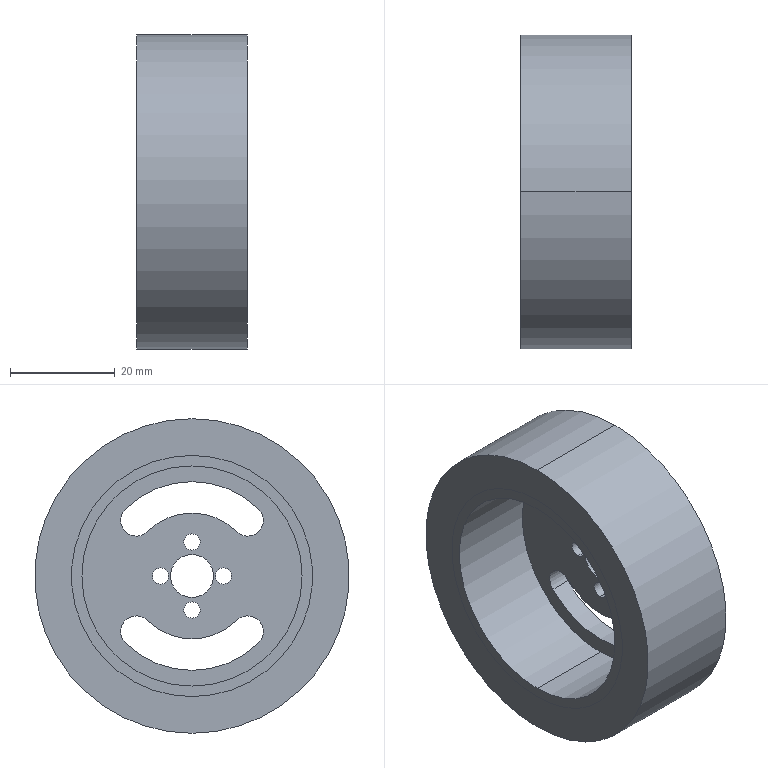Part | SolidWorks | features BaseBody 2 | 2 solids | 35 faces | box 21 x 60 x 60 mm | volume 34134 mm3 | cylinder 30 | plane 5 | commonest cylinder face diameters 3.1 x8 6 x6 46 x4 24 x3 36 x3 8.2 x2
STEP:
#1=CARTESIAN_POINT('',(39.982,27.528,21.886));
#2=VERTEX_POINT('',#1);
#3=CARTESIAN_POINT('',(18.982,27.528,21.886));
#4=VERTEX_POINT('',#3);
#5=CARTESIAN_POINT('',(39.982,27.528,21.886));
#6=DIRECTION('',(-1.,0.,0.));
#7=VECTOR('',#6,1000.);
#8=LINE('',#5,#7);
#9=EDGE_CURVE('',#2,#4,#8,.T.);
#10=ORIENTED_EDGE('',*,*,#9,.F.);
#11=CARTESIAN_POINT('',(39.982,27.528,67.886));
#12=VERTEX_POINT('',#11);
#13=CARTESIAN_POINT('',(39.982,27.528,44.886));
#14=DIRECTION('',(1.,0.,0.));
#15=DIRECTION('',(0.,0.,-1.));
#16=AXIS2_PLACEMENT_3D('',#13,#14,#15);
#17=CIRCLE('',#16,23.);
#18=EDGE_CURVE('',#2,#12,#17,.T.);
#19=ORIENTED_EDGE('',*,*,#18,.T.);
#20=CARTESIAN_POINT('',(18.982,27.528,67.886));
#21=VERTEX_POINT('',#20);
#22=CARTESIAN_POINT('',(39.982,27.528,67.886));
#23=DIRECTION('',(-1.,0.,0.));
#24=VECTOR('',#23,1000.);
#25=LINE('',#22,#24);
#26=EDGE_CURVE('',#12,#21,#25,.T.);
#27=ORIENTED_EDGE('',*,*,#26,.T.);
#28=CARTESIAN_POINT('',(18.982,27.528,44.886));
#29=DIRECTION('',(1.,0.,0.));
#30=DIRECTION('',(0.,0.,-1.));
#31=AXIS2_PLACEMENT_3D('',#28,#29,#30);
#32=CIRCLE('',#31,23.);
#33=EDGE_CURVE('',#4,#21,#32,.T.);
#34=ORIENTED_EDGE('',*,*,#33,.F.);
#35=EDGE_LOOP('',(#10,#19,#27,#34));
#36=FACE_OUTER_BOUND('',#35,.T.);
#37=CARTESIAN_POINT('',(39.982,27.528,44.886));
#38=DIRECTION('',(-1.,0.,0.));
#39=DIRECTION('',(0.,0.,1.));
#40=AXIS2_PLACEMENT_3D('',#37,#38,#39);
#41=CYLINDRICAL_SURFACE('',#40,23.);
#42=ADVANCED_FACE('',(#36),#41,.F.);
#43=CARTESIAN_POINT('',(39.982,27.528,14.886));
#44=VERTEX_POINT('',#43);
#45=CARTESIAN_POINT('',(18.982,27.528,14.886));
#46=VERTEX_POINT('',#45);
#47=CARTESIAN_POINT('',(39.982,27.528,14.886));
#48=DIRECTION('',(-1.,0.,0.));
#49=VECTOR('',#48,1000.);
#50=LINE('',#47,#49);
#51=EDGE_CURVE('',#44,#46,#50,.T.);
#52=ORIENTED_EDGE('',*,*,#51,.F.);
#53=CARTESIAN_POINT('',(39.982,27.528,74.886));
#54=VERTEX_POINT('',#53);
#55=CARTESIAN_POINT('',(39.982,27.528,44.886));
#56=DIRECTION('',(1.,0.,0.));
#57=DIRECTION('',(0.,0.,-1.));
#58=AXIS2_PLACEMENT_3D('',#55,#56,#57);
#59=CIRCLE('',#58,30.);
#60=EDGE_CURVE('',#54,#44,#59,.T.);
#61=ORIENTED_EDGE('',*,*,#60,.F.);
#62=CARTESIAN_POINT('',(18.982,27.528,74.886));
#63=VERTEX_POINT('',#62);
#64=CARTESIAN_POINT('',(39.982,27.528,74.886));
#65=DIRECTION('',(-1.,0.,0.));
#66=VECTOR('',#65,1000.);
#67=LINE('',#64,#66);
#68=EDGE_CURVE('',#54,#63,#67,.T.);
#69=ORIENTED_EDGE('',*,*,#68,.T.);
#70=CARTESIAN_POINT('',(18.982,27.528,44.886));
#71=DIRECTION('',(1.,0.,0.));
#72=DIRECTION('',(0.,0.,-1.));
#73=AXIS2_PLACEMENT_3D('',#70,#71,#72);
#74=CIRCLE('',#73,30.);
#75=EDGE_CURVE('',#63,#46,#74,.T.);
#76=ORIENTED_EDGE('',*,*,#75,.T.);
#77=EDGE_LOOP('',(#52,#61,#69,#76));
#78=FACE_OUTER_BOUND('',#77,.T.);
#79=CARTESIAN_POINT('',(39.982,27.528,44.886));
#80=DIRECTION('',(-1.,0.,0.));
#81=DIRECTION('',(0.,0.,1.));
#82=AXIS2_PLACEMENT_3D('',#79,#80,#81);
#83=CYLINDRICAL_SURFACE('',#82,30.);
#84=ADVANCED_FACE('',(#78),#83,.T.);
#85=CARTESIAN_POINT('',(18.982,27.528,44.886));
#86=DIRECTION('',(1.,0.,0.));
#87=DIRECTION('',(0.,0.,-1.));
#88=AXIS2_PLACEMENT_3D('',#85,#86,#87);
#89=CIRCLE('',#88,23.);
#90=EDGE_CURVE('',#21,#4,#89,.T.);
#91=ORIENTED_EDGE('',*,*,#90,.T.);
#92=ORIENTED_EDGE('',*,*,#33,.T.);
#93=EDGE_LOOP('',(#91,#92));
#94=FACE_BOUND('',#93,.T.);
#95=ORIENTED_EDGE('',*,*,#75,.F.);
#96=CARTESIAN_POINT('',(18.982,27.528,44.886));
#97=DIRECTION('',(1.,0.,0.));
#98=DIRECTION('',(0.,0.,-1.));
#99=AXIS2_PLACEMENT_3D('',#96,#97,#98);
#100=CIRCLE('',#99,30.);
#101=EDGE_CURVE('',#46,#63,#100,.T.);
#102=ORIENTED_EDGE('',*,*,#101,.F.);
#103=EDGE_LOOP('',(#95,#102));
#104=FACE_OUTER_BOUND('',#103,.T.);
#105=CARTESIAN_POINT('',(18.982,27.528,44.886));
#106=DIRECTION('',(1.,0.,0.));
#107=DIRECTION('',(0.,1.,0.));
#108=AXIS2_PLACEMENT_3D('',#105,#106,#107);
#109=PLANE('',#108);
#110=ADVANCED_FACE('',(#94,#104),#109,.F.);
#111=CARTESIAN_POINT('',(39.982,27.528,44.886));
#112=DIRECTION('',(1.,0.,0.));
#113=DIRECTION('',(0.,0.,-1.));
#114=AXIS2_PLACEMENT_3D('',#111,#112,#113);
#115=CIRCLE('',#114,23.);
#116=EDGE_CURVE('',#12,#2,#115,.T.);
#117=ORIENTED_EDGE('',*,*,#116,.F.);
#118=ORIENTED_EDGE('',*,*,#18,.F.);
#119=EDGE_LOOP('',(#117,#118));
#120=FACE_BOUND('',#119,.T.);
#121=ORIENTED_EDGE('',*,*,#60,.T.);
#122=CARTESIAN_POINT('',(39.982,27.528,44.886));
#123=DIRECTION('',(1.,0.,0.));
#124=DIRECTION('',(0.,0.,-1.));
#125=AXIS2_PLACEMENT_3D('',#122,#123,#124);
#126=CIRCLE('',#125,30.);
#127=EDGE_CURVE('',#44,#54,#126,.T.);
#128=ORIENTED_EDGE('',*,*,#127,.T.);
#129=EDGE_LOOP('',(#121,#128));
#130=FACE_OUTER_BOUND('',#129,.T.);
#131=CARTESIAN_POINT('',(39.982,27.528,44.886));
#132=DIRECTION('',(1.,0.,0.));
#133=DIRECTION('',(0.,1.,0.));
#134=AXIS2_PLACEMENT_3D('',#131,#132,#133);
#135=PLANE('',#134);
#136=ADVANCED_FACE('',(#120,#130),#135,.T.);
#137=ORIENTED_EDGE('',*,*,#127,.F.);
#138=ORIENTED_EDGE('',*,*,#51,.T.);
#139=ORIENTED_EDGE('',*,*,#101,.T.);
#140=ORIENTED_EDGE('',*,*,#68,.F.);
#141=EDGE_LOOP('',(#137,#138,#139,#140));
#142=FACE_OUTER_BOUND('',#141,.T.);
#143=CARTESIAN_POINT('',(39.982,27.528,44.886));
#144=DIRECTION('',(-1.,0.,0.));
#145=DIRECTION('',(0.,0.,1.));
#146=AXIS2_PLACEMENT_3D('',#143,#144,#145);
#147=CYLINDRICAL_SURFACE('',#146,30.);
#148=ADVANCED_FACE('',(#142),#147,.T.);
#149=ORIENTED_EDGE('',*,*,#116,.T.);
#150=ORIENTED_EDGE('',*,*,#9,.T.);
#151=ORIENTED_EDGE('',*,*,#90,.F.);
#152=ORIENTED_EDGE('',*,*,#26,.F.);
#153=EDGE_LOOP('',(#149,#150,#151,#152));
#154=FACE_OUTER_BOUND('',#153,.T.);
#155=CARTESIAN_POINT('',(39.982,27.528,44.886));
#156=DIRECTION('',(-1.,0.,0.));
#157=DIRECTION('',(0.,0.,1.));
#158=AXIS2_PLACEMENT_3D('',#155,#156,#157);
#159=CYLINDRICAL_SURFACE('',#158,23.);
#160=ADVANCED_FACE('',(#154),#159,.F.);
#161=CLOSED_SHELL('',(#42,#84,#110,#136,#148,#160));
#162=MANIFOLD_SOLID_BREP('',#161);
#163=CARTESIAN_POINT('',(35.982,27.528,39.936));
#164=VERTEX_POINT('',#163);
#165=CARTESIAN_POINT('',(35.982,27.528,36.836));
#166=VERTEX_POINT('',#165);
#167=CARTESIAN_POINT('',(35.982,27.528,38.386));
#168=DIRECTION('',(-1.,0.,0.));
#169=DIRECTION('',(0.,0.,1.));
#170=AXIS2_PLACEMENT_3D('',#167,#168,#169);
#171=CIRCLE('',#170,1.55);
#172=EDGE_CURVE('',#164,#166,#171,.T.);
#173=ORIENTED_EDGE('',*,*,#172,.F.);
#174=CARTESIAN_POINT('',(35.982,27.528,38.386));
#175=DIRECTION('',(-1.,0.,0.));
#176=DIRECTION('',(0.,0.,1.));
#177=AXIS2_PLACEMENT_3D('',#174,#175,#176);
#178=CIRCLE('',#177,1.55);
#179=EDGE_CURVE('',#166,#164,#178,.T.);
#180=ORIENTED_EDGE('',*,*,#179,.F.);
#181=EDGE_LOOP('',(#173,#180));
#182=FACE_BOUND('',#181,.T.);
#183=CARTESIAN_POINT('',(35.982,21.528,46.436));
#184=VERTEX_POINT('',#183);
#185=CARTESIAN_POINT('',(35.982,21.528,43.336));
#186=VERTEX_POINT('',#185);
#187=CARTESIAN_POINT('',(35.982,21.528,44.886));
#188=DIRECTION('',(-1.,0.,0.));
#189=DIRECTION('',(0.,0.,-1.));
#190=AXIS2_PLACEMENT_3D('',#187,#188,#189);
#191=CIRCLE('',#190,1.55);
#192=EDGE_CURVE('',#184,#186,#191,.T.);
#193=ORIENTED_EDGE('',*,*,#192,.F.);
#194=CARTESIAN_POINT('',(35.982,21.528,44.886));
#195=DIRECTION('',(-1.,0.,0.));
#196=DIRECTION('',(0.,0.,-1.));
#197=AXIS2_PLACEMENT_3D('',#194,#195,#196);
#198=CIRCLE('',#197,1.55);
#199=EDGE_CURVE('',#186,#184,#198,.T.);
#200=ORIENTED_EDGE('',*,*,#199,.F.);
#201=EDGE_LOOP('',(#193,#200));
#202=FACE_BOUND('',#201,.T.);
#203=CARTESIAN_POINT('',(35.982,27.528,52.936));
#204=VERTEX_POINT('',#203);
#205=CARTESIAN_POINT('',(35.982,27.528,49.836));
#206=VERTEX_POINT('',#205);
#207=CARTESIAN_POINT('',(35.982,27.528,51.386));
#208=DIRECTION('',(-1.,0.,0.));
#209=DIRECTION('',(0.,0.,-1.));
#210=AXIS2_PLACEMENT_3D('',#207,#208,#209);
#211=CIRCLE('',#210,1.55);
#212=EDGE_CURVE('',#204,#206,#211,.T.);
#213=ORIENTED_EDGE('',*,*,#212,.F.);
#214=CARTESIAN_POINT('',(35.982,27.528,51.386));
#215=DIRECTION('',(-1.,0.,0.));
#216=DIRECTION('',(0.,0.,-1.));
#217=AXIS2_PLACEMENT_3D('',#214,#215,#216);
#218=CIRCLE('',#217,1.55);
#219=EDGE_CURVE('',#206,#204,#218,.T.);
#220=ORIENTED_EDGE('',*,*,#219,.F.);
#221=EDGE_LOOP('',(#213,#220));
#222=FACE_BOUND('',#221,.T.);
#223=CARTESIAN_POINT('',(35.982,33.528,46.436));
#224=VERTEX_POINT('',#223);
#225=CARTESIAN_POINT('',(35.982,33.528,43.336));
#226=VERTEX_POINT('',#225);
#227=CARTESIAN_POINT('',(35.982,33.528,44.886));
#228=DIRECTION('',(-1.,0.,0.));
#229=DIRECTION('',(0.,0.,1.));
#230=AXIS2_PLACEMENT_3D('',#227,#228,#229);
#231=CIRCLE('',#230,1.55);
#232=EDGE_CURVE('',#224,#226,#231,.T.);
#233=ORIENTED_EDGE('',*,*,#232,.F.);
#234=CARTESIAN_POINT('',(35.982,33.528,44.886));
#235=DIRECTION('',(-1.,0.,0.));
#236=DIRECTION('',(0.,0.,1.));
#237=AXIS2_PLACEMENT_3D('',#234,#235,#236);
#238=CIRCLE('',#237,1.55);
#239=EDGE_CURVE('',#226,#224,#238,.T.);
#240=ORIENTED_EDGE('',*,*,#239,.F.);
#241=EDGE_LOOP('',(#233,#240));
#242=FACE_BOUND('',#241,.T.);
#243=CARTESIAN_POINT('',(35.982,27.528,48.986));
#244=VERTEX_POINT('',#243);
#245=CARTESIAN_POINT('',(35.982,27.528,40.786));
#246=VERTEX_POINT('',#245);
#247=CARTESIAN_POINT('',(35.982,27.528,44.886));
#248=DIRECTION('',(-1.,0.,0.));
#249=DIRECTION('',(0.,0.,-1.));
#250=AXIS2_PLACEMENT_3D('',#247,#248,#249);
#251=CIRCLE('',#250,4.1);
#252=EDGE_CURVE('',#244,#246,#251,.T.);
#253=ORIENTED_EDGE('',*,*,#252,.F.);
#254=CARTESIAN_POINT('',(35.982,27.528,44.886));
#255=DIRECTION('',(-1.,0.,0.));
#256=DIRECTION('',(0.,0.,-1.));
#257=AXIS2_PLACEMENT_3D('',#254,#255,#256);
#258=CIRCLE('',#257,4.1);
#259=EDGE_CURVE('',#246,#244,#258,.T.);
#260=ORIENTED_EDGE('',*,*,#259,.F.);
#261=EDGE_LOOP('',(#253,#260));
#262=FACE_BOUND('',#261,.T.);
#263=CARTESIAN_POINT('',(35.982,19.043,36.401));
#264=VERTEX_POINT('',#263);
#265=CARTESIAN_POINT('',(35.982,36.014,36.401));
#266=VERTEX_POINT('',#265);
#267=CARTESIAN_POINT('',(35.982,27.528,44.886));
#268=DIRECTION('',(1.,0.,0.));
#269=DIRECTION('',(0.,0.,-1.));
#270=AXIS2_PLACEMENT_3D('',#267,#268,#269);
#271=CIRCLE('',#270,12.);
#272=EDGE_CURVE('',#264,#266,#271,.T.);
#273=ORIENTED_EDGE('',*,*,#272,.F.);
#274=CARTESIAN_POINT('',(35.982,16.922,37.28));
#275=VERTEX_POINT('',#274);
#276=CARTESIAN_POINT('',(35.982,16.922,34.28));
#277=DIRECTION('',(-1.,0.,0.));
#278=DIRECTION('',(0.,0.,-1.));
#279=AXIS2_PLACEMENT_3D('',#276,#277,#278);
#280=CIRCLE('',#279,3.);
#281=EDGE_CURVE('',#275,#264,#280,.T.);
#282=ORIENTED_EDGE('',*,*,#281,.F.);
#283=CARTESIAN_POINT('',(35.982,14.801,32.158));
#284=VERTEX_POINT('',#283);
#285=CARTESIAN_POINT('',(35.982,16.922,34.28));
#286=DIRECTION('',(-1.,0.,0.));
#287=DIRECTION('',(0.,0.,-1.));
#288=AXIS2_PLACEMENT_3D('',#285,#286,#287);
#289=CIRCLE('',#288,3.);
#290=EDGE_CURVE('',#284,#275,#289,.T.);
#291=ORIENTED_EDGE('',*,*,#290,.F.);
#292=CARTESIAN_POINT('',(35.982,40.256,32.158));
#293=VERTEX_POINT('',#292);
#294=CARTESIAN_POINT('',(35.982,27.528,44.886));
#295=DIRECTION('',(-1.,0.,0.));
#296=DIRECTION('',(0.,0.,-1.));
#297=AXIS2_PLACEMENT_3D('',#294,#295,#296);
#298=CIRCLE('',#297,18.);
#299=EDGE_CURVE('',#293,#284,#298,.T.);
#300=ORIENTED_EDGE('',*,*,#299,.F.);
#301=CARTESIAN_POINT('',(35.982,38.135,37.28));
#302=VERTEX_POINT('',#301);
#303=CARTESIAN_POINT('',(35.982,38.135,34.28));
#304=DIRECTION('',(-1.,0.,0.));
#305=DIRECTION('',(0.,0.,-1.));
#306=AXIS2_PLACEMENT_3D('',#303,#304,#305);
#307=CIRCLE('',#306,3.);
#308=EDGE_CURVE('',#302,#293,#307,.T.);
#309=ORIENTED_EDGE('',*,*,#308,.F.);
#310=CARTESIAN_POINT('',(35.982,38.135,34.28));
#311=DIRECTION('',(-1.,0.,0.));
#312=DIRECTION('',(0.,0.,-1.));
#313=AXIS2_PLACEMENT_3D('',#310,#311,#312);
#314=CIRCLE('',#313,3.);
#315=EDGE_CURVE('',#266,#302,#314,.T.);
#316=ORIENTED_EDGE('',*,*,#315,.F.);
#317=EDGE_LOOP('',(#273,#282,#291,#300,#309,#316));
#318=FACE_BOUND('',#317,.T.);
#319=CARTESIAN_POINT('',(35.982,19.043,53.372));
#320=VERTEX_POINT('',#319);
#321=CARTESIAN_POINT('',(35.982,14.801,57.614));
#322=VERTEX_POINT('',#321);
#323=CARTESIAN_POINT('',(35.982,16.922,55.493));
#324=DIRECTION('',(-1.,0.,0.));
#325=DIRECTION('',(0.,0.,1.));
#326=AXIS2_PLACEMENT_3D('',#323,#324,#325);
#327=CIRCLE('',#326,3.);
#328=EDGE_CURVE('',#320,#322,#327,.T.);
#329=ORIENTED_EDGE('',*,*,#328,.F.);
#330=CARTESIAN_POINT('',(35.982,27.528,56.886));
#331=VERTEX_POINT('',#330);
#332=CARTESIAN_POINT('',(35.982,27.528,44.886));
#333=DIRECTION('',(1.,0.,0.));
#334=DIRECTION('',(0.,0.,1.));
#335=AXIS2_PLACEMENT_3D('',#332,#333,#334);
#336=CIRCLE('',#335,12.);
#337=EDGE_CURVE('',#331,#320,#336,.T.);
#338=ORIENTED_EDGE('',*,*,#337,.F.);
#339=CARTESIAN_POINT('',(35.982,36.014,53.372));
#340=VERTEX_POINT('',#339);
#341=CARTESIAN_POINT('',(35.982,27.528,44.886));
#342=DIRECTION('',(1.,0.,0.));
#343=DIRECTION('',(0.,0.,1.));
#344=AXIS2_PLACEMENT_3D('',#341,#342,#343);
#345=CIRCLE('',#344,12.);
#346=EDGE_CURVE('',#340,#331,#345,.T.);
#347=ORIENTED_EDGE('',*,*,#346,.F.);
#348=CARTESIAN_POINT('',(35.982,40.256,57.614));
#349=VERTEX_POINT('',#348);
#350=CARTESIAN_POINT('',(35.982,38.135,55.493));
#351=DIRECTION('',(-1.,0.,0.));
#352=DIRECTION('',(0.,0.,1.));
#353=AXIS2_PLACEMENT_3D('',#350,#351,#352);
#354=CIRCLE('',#353,3.);
#355=EDGE_CURVE('',#349,#340,#354,.T.);
#356=ORIENTED_EDGE('',*,*,#355,.F.);
#357=CARTESIAN_POINT('',(35.982,27.528,62.886));
#358=VERTEX_POINT('',#357);
#359=CARTESIAN_POINT('',(35.982,27.528,44.886));
#360=DIRECTION('',(-1.,0.,0.));
#361=DIRECTION('',(0.,0.,1.));
#362=AXIS2_PLACEMENT_3D('',#359,#360,#361);
#363=CIRCLE('',#362,18.);
#364=EDGE_CURVE('',#358,#349,#363,.T.);
#365=ORIENTED_EDGE('',*,*,#364,.F.);
#366=CARTESIAN_POINT('',(35.982,27.528,44.886));
#367=DIRECTION('',(-1.,0.,0.));
#368=DIRECTION('',(0.,0.,1.));
#369=AXIS2_PLACEMENT_3D('',#366,#367,#368);
#370=CIRCLE('',#369,18.);
#371=EDGE_CURVE('',#322,#358,#370,.T.);
#372=ORIENTED_EDGE('',*,*,#371,.F.);
#373=EDGE_LOOP('',(#329,#338,#347,#356,#365,#372));
#374=FACE_BOUND('',#373,.T.);
#375=CARTESIAN_POINT('',(35.982,27.528,65.886));
#376=VERTEX_POINT('',#375);
#377=CARTESIAN_POINT('',(35.982,27.528,23.886));
#378=VERTEX_POINT('',#377);
#379=CARTESIAN_POINT('',(35.982,27.528,44.886));
#380=DIRECTION('',(-1.,0.,0.));
#381=DIRECTION('',(0.,0.,-1.));
#382=AXIS2_PLACEMENT_3D('',#379,#380,#381);
#383=CIRCLE('',#382,21.);
#384=EDGE_CURVE('',#376,#378,#383,.T.);
#385=ORIENTED_EDGE('',*,*,#384,.T.);
#386=CARTESIAN_POINT('',(35.982,27.528,44.886));
#387=DIRECTION('',(-1.,0.,0.));
#388=DIRECTION('',(0.,0.,-1.));
#389=AXIS2_PLACEMENT_3D('',#386,#387,#388);
#390=CIRCLE('',#389,21.);
#391=EDGE_CURVE('',#378,#376,#390,.T.);
#392=ORIENTED_EDGE('',*,*,#391,.T.);
#393=EDGE_LOOP('',(#385,#392));
#394=FACE_OUTER_BOUND('',#393,.T.);
#395=CARTESIAN_POINT('',(35.982,27.528,44.886));
#396=DIRECTION('',(-1.,0.,0.));
#397=DIRECTION('',(0.,-1.,0.));
#398=AXIS2_PLACEMENT_3D('',#395,#396,#397);
#399=PLANE('',#398);
#400=ADVANCED_FACE('',(#182,#202,#222,#242,#262,#318,#374,#394),#399,.T.);
#401=CARTESIAN_POINT('',(18.982,27.528,23.886));
#402=VERTEX_POINT('',#401);
#403=CARTESIAN_POINT('',(18.982,27.528,23.886));
#404=DIRECTION('',(1.,0.,0.));
#405=VECTOR('',#404,1000.);
#406=LINE('',#403,#405);
#407=EDGE_CURVE('',#402,#378,#406,.T.);
#408=ORIENTED_EDGE('',*,*,#407,.F.);
#409=CARTESIAN_POINT('',(18.982,27.528,65.886));
#410=VERTEX_POINT('',#409);
#411=CARTESIAN_POINT('',(18.982,27.528,44.886));
#412=DIRECTION('',(-1.,0.,0.));
#413=DIRECTION('',(0.,0.,-1.));
#414=AXIS2_PLACEMENT_3D('',#411,#412,#413);
#415=CIRCLE('',#414,21.);
#416=EDGE_CURVE('',#402,#410,#415,.T.);
#417=ORIENTED_EDGE('',*,*,#416,.T.);
#418=CARTESIAN_POINT('',(18.982,27.528,65.886));
#419=DIRECTION('',(1.,0.,0.));
#420=VECTOR('',#419,1000.);
#421=LINE('',#418,#420);
#422=EDGE_CURVE('',#410,#376,#421,.T.);
#423=ORIENTED_EDGE('',*,*,#422,.T.);
#424=ORIENTED_EDGE('',*,*,#391,.F.);
#425=EDGE_LOOP('',(#408,#417,#423,#424));
#426=FACE_OUTER_BOUND('',#425,.T.);
#427=CARTESIAN_POINT('',(18.982,27.528,44.886));
#428=DIRECTION('',(1.,0.,0.));
#429=DIRECTION('',(0.,0.,1.));
#430=AXIS2_PLACEMENT_3D('',#427,#428,#429);
#431=CYLINDRICAL_SURFACE('',#430,21.);
#432=ADVANCED_FACE('',(#426),#431,.F.);
#433=CARTESIAN_POINT('',(18.982,27.528,44.886));
#434=DIRECTION('',(-1.,0.,0.));
#435=DIRECTION('',(0.,0.,-1.));
#436=AXIS2_PLACEMENT_3D('',#433,#434,#435);
#437=CIRCLE('',#436,21.);
#438=EDGE_CURVE('',#410,#402,#437,.T.);
#439=ORIENTED_EDGE('',*,*,#438,.F.);
#440=ORIENTED_EDGE('',*,*,#416,.F.);
#441=EDGE_LOOP('',(#439,#440));
#442=FACE_BOUND('',#441,.T.);
#443=CARTESIAN_POINT('',(18.982,27.528,67.886));
#444=VERTEX_POINT('',#443);
#445=CARTESIAN_POINT('',(18.982,27.528,21.886));
#446=VERTEX_POINT('',#445);
#447=CARTESIAN_POINT('',(18.982,27.528,44.886));
#448=DIRECTION('',(-1.,0.,0.));
#449=DIRECTION('',(0.,0.,-1.));
#450=AXIS2_PLACEMENT_3D('',#447,#448,#449);
#451=CIRCLE('',#450,23.);
#452=EDGE_CURVE('',#444,#446,#451,.T.);
#453=ORIENTED_EDGE('',*,*,#452,.T.);
#454=CARTESIAN_POINT('',(18.982,27.528,44.886));
#455=DIRECTION('',(-1.,0.,0.));
#456=DIRECTION('',(0.,0.,-1.));
#457=AXIS2_PLACEMENT_3D('',#454,#455,#456);
#458=CIRCLE('',#457,23.);
#459=EDGE_CURVE('',#446,#444,#458,.T.);
#460=ORIENTED_EDGE('',*,*,#459,.T.);
#461=EDGE_LOOP('',(#453,#460));
#462=FACE_OUTER_BOUND('',#461,.T.);
#463=CARTESIAN_POINT('',(18.982,27.528,44.886));
#464=DIRECTION('',(-1.,0.,0.));
#465=DIRECTION('',(0.,-1.,0.));
#466=AXIS2_PLACEMENT_3D('',#463,#464,#465);
#467=PLANE('',#466);
#468=ADVANCED_FACE('',(#442,#462),#467,.T.);
#469=CARTESIAN_POINT('',(39.982,40.256,57.614));
#470=VERTEX_POINT('',#469);
#471=CARTESIAN_POINT('',(39.982,36.014,53.372));
#472=VERTEX_POINT('',#471);
#473=CARTESIAN_POINT('',(39.982,38.135,55.493));
#474=DIRECTION('',(-1.,0.,0.));
#475=DIRECTION('',(0.,0.,1.));
#476=AXIS2_PLACEMENT_3D('',#473,#474,#475);
#477=CIRCLE('',#476,3.);
#478=EDGE_CURVE('',#470,#472,#477,.T.);
#479=ORIENTED_EDGE('',*,*,#478,.F.);
#480=CARTESIAN_POINT('',(37.982,40.256,57.614));
#481=DIRECTION('',(1.,0.,0.));
#482=VECTOR('',#481,1000.);
#483=LINE('',#480,#482);
#484=EDGE_CURVE('',#349,#470,#483,.T.);
#485=ORIENTED_EDGE('',*,*,#484,.F.);
#486=ORIENTED_EDGE('',*,*,#355,.T.);
#487=CARTESIAN_POINT('',(37.982,36.014,53.372));
#488=DIRECTION('',(1.,0.,0.));
#489=VECTOR('',#488,1000.);
#490=LINE('',#487,#489);
#491=EDGE_CURVE('',#340,#472,#490,.T.);
#492=ORIENTED_EDGE('',*,*,#491,.T.);
#493=EDGE_LOOP('',(#479,#485,#486,#492));
#494=FACE_OUTER_BOUND('',#493,.T.);
#495=CARTESIAN_POINT('',(37.982,38.135,55.493));
#496=DIRECTION('',(1.,0.,0.));
#497=DIRECTION('',(0.,0.,1.));
#498=AXIS2_PLACEMENT_3D('',#495,#496,#497);
#499=CYLINDRICAL_SURFACE('',#498,3.);
#500=ADVANCED_FACE('',(#494),#499,.F.);
#501=CARTESIAN_POINT('',(39.982,27.528,62.886));
#502=VERTEX_POINT('',#501);
#503=CARTESIAN_POINT('',(37.982,27.528,62.886));
#504=DIRECTION('',(1.,0.,0.));
#505=VECTOR('',#504,1000.);
#506=LINE('',#503,#505);
#507=EDGE_CURVE('',#358,#502,#506,.T.);
#508=ORIENTED_EDGE('',*,*,#507,.F.);
#509=ORIENTED_EDGE('',*,*,#364,.T.);
#510=ORIENTED_EDGE('',*,*,#484,.T.);
#511=CARTESIAN_POINT('',(39.982,27.528,44.886));
#512=DIRECTION('',(-1.,0.,0.));
#513=DIRECTION('',(0.,0.,1.));
#514=AXIS2_PLACEMENT_3D('',#511,#512,#513);
#515=CIRCLE('',#514,18.);
#516=EDGE_CURVE('',#502,#470,#515,.T.);
#517=ORIENTED_EDGE('',*,*,#516,.F.);
#518=EDGE_LOOP('',(#508,#509,#510,#517));
#519=FACE_OUTER_BOUND('',#518,.T.);
#520=CARTESIAN_POINT('',(37.982,27.528,44.886));
#521=DIRECTION('',(1.,0.,0.));
#522=DIRECTION('',(0.,0.,1.));
#523=AXIS2_PLACEMENT_3D('',#520,#521,#522);
#524=CYLINDRICAL_SURFACE('',#523,18.);
#525=ADVANCED_FACE('',(#519),#524,.F.);
#526=CARTESIAN_POINT('',(39.982,19.043,53.372));
#527=VERTEX_POINT('',#526);
#528=CARTESIAN_POINT('',(39.982,14.801,57.614));
#529=VERTEX_POINT('',#528);
#530=CARTESIAN_POINT('',(39.982,16.922,55.493));
#531=DIRECTION('',(-1.,0.,0.));
#532=DIRECTION('',(0.,0.,1.));
#533=AXIS2_PLACEMENT_3D('',#530,#531,#532);
#534=CIRCLE('',#533,3.);
#535=EDGE_CURVE('',#527,#529,#534,.T.);
#536=ORIENTED_EDGE('',*,*,#535,.F.);
#537=CARTESIAN_POINT('',(37.982,19.043,53.372));
#538=DIRECTION('',(1.,0.,0.));
#539=VECTOR('',#538,1000.);
#540=LINE('',#537,#539);
#541=EDGE_CURVE('',#320,#527,#540,.T.);
#542=ORIENTED_EDGE('',*,*,#541,.F.);
#543=ORIENTED_EDGE('',*,*,#328,.T.);
#544=CARTESIAN_POINT('',(37.982,14.801,57.614));
#545=DIRECTION('',(1.,0.,0.));
#546=VECTOR('',#545,1000.);
#547=LINE('',#544,#546);
#548=EDGE_CURVE('',#322,#529,#547,.T.);
#549=ORIENTED_EDGE('',*,*,#548,.T.);
#550=EDGE_LOOP('',(#536,#542,#543,#549));
#551=FACE_OUTER_BOUND('',#550,.T.);
#552=CARTESIAN_POINT('',(37.982,16.922,55.493));
#553=DIRECTION('',(1.,0.,0.));
#554=DIRECTION('',(0.,0.,1.));
#555=AXIS2_PLACEMENT_3D('',#552,#553,#554);
#556=CYLINDRICAL_SURFACE('',#555,3.);
#557=ADVANCED_FACE('',(#551),#556,.F.);
#558=CARTESIAN_POINT('',(39.982,27.528,56.886));
#559=VERTEX_POINT('',#558);
#560=CARTESIAN_POINT('',(37.982,27.528,56.886));
#561=DIRECTION('',(1.,0.,0.));
#562=VECTOR('',#561,1000.);
#563=LINE('',#560,#562);
#564=EDGE_CURVE('',#331,#559,#563,.T.);
#565=ORIENTED_EDGE('',*,*,#564,.F.);
#566=ORIENTED_EDGE('',*,*,#337,.T.);
#567=ORIENTED_EDGE('',*,*,#541,.T.);
#568=CARTESIAN_POINT('',(39.982,27.528,44.886));
#569=DIRECTION('',(1.,0.,0.));
#570=DIRECTION('',(0.,0.,1.));
#571=AXIS2_PLACEMENT_3D('',#568,#569,#570);
#572=CIRCLE('',#571,12.);
#573=EDGE_CURVE('',#559,#527,#572,.T.);
#574=ORIENTED_EDGE('',*,*,#573,.F.);
#575=EDGE_LOOP('',(#565,#566,#567,#574));
#576=FACE_OUTER_BOUND('',#575,.T.);
#577=CARTESIAN_POINT('',(37.982,27.528,44.886));
#578=DIRECTION('',(1.,0.,0.));
#579=DIRECTION('',(0.,0.,1.));
#580=AXIS2_PLACEMENT_3D('',#577,#578,#579);
#581=CYLINDRICAL_SURFACE('',#580,12.);
#582=ADVANCED_FACE('',(#576),#581,.T.);
#583=CARTESIAN_POINT('',(39.982,40.256,32.158));
#584=VERTEX_POINT('',#583);
#585=CARTESIAN_POINT('',(39.982,14.801,32.158));
#586=VERTEX_POINT('',#585);
#587=CARTESIAN_POINT('',(39.982,27.528,44.886));
#588=DIRECTION('',(-1.,0.,0.));
#589=DIRECTION('',(0.,0.,-1.));
#590=AXIS2_PLACEMENT_3D('',#587,#588,#589);
#591=CIRCLE('',#590,18.);
#592=EDGE_CURVE('',#584,#586,#591,.T.);
#593=ORIENTED_EDGE('',*,*,#592,.F.);
#594=CARTESIAN_POINT('',(37.982,40.256,32.158));
#595=DIRECTION('',(1.,0.,0.));
#596=VECTOR('',#595,1000.);
#597=LINE('',#594,#596);
#598=EDGE_CURVE('',#293,#584,#597,.T.);
#599=ORIENTED_EDGE('',*,*,#598,.F.);
#600=ORIENTED_EDGE('',*,*,#299,.T.);
#601=CARTESIAN_POINT('',(37.982,14.801,32.158));
#602=DIRECTION('',(1.,0.,0.));
#603=VECTOR('',#602,1000.);
#604=LINE('',#601,#603);
#605=EDGE_CURVE('',#284,#586,#604,.T.);
#606=ORIENTED_EDGE('',*,*,#605,.T.);
#607=EDGE_LOOP('',(#593,#599,#600,#606));
#608=FACE_OUTER_BOUND('',#607,.T.);
#609=CARTESIAN_POINT('',(37.982,27.528,44.886));
#610=DIRECTION('',(1.,0.,0.));
#611=DIRECTION('',(0.,0.,1.));
#612=AXIS2_PLACEMENT_3D('',#609,#610,#611);
#613=CYLINDRICAL_SURFACE('',#612,18.);
#614=ADVANCED_FACE('',(#608),#613,.F.);
#615=CARTESIAN_POINT('',(39.982,38.135,37.28));
#616=VERTEX_POINT('',#615);
#617=CARTESIAN_POINT('',(37.982,38.135,37.28));
#618=DIRECTION('',(1.,0.,0.));
#619=VECTOR('',#618,1000.);
#620=LINE('',#617,#619);
#621=EDGE_CURVE('',#302,#616,#620,.T.);
#622=ORIENTED_EDGE('',*,*,#621,.F.);
#623=ORIENTED_EDGE('',*,*,#308,.T.);
#624=ORIENTED_EDGE('',*,*,#598,.T.);
#625=CARTESIAN_POINT('',(39.982,38.135,34.28));
#626=DIRECTION('',(-1.,0.,0.));
#627=DIRECTION('',(0.,0.,-1.));
#628=AXIS2_PLACEMENT_3D('',#625,#626,#627);
#629=CIRCLE('',#628,3.);
#630=EDGE_CURVE('',#616,#584,#629,.T.);
#631=ORIENTED_EDGE('',*,*,#630,.F.);
#632=EDGE_LOOP('',(#622,#623,#624,#631));
#633=FACE_OUTER_BOUND('',#632,.T.);
#634=CARTESIAN_POINT('',(37.982,38.135,34.28));
#635=DIRECTION('',(1.,0.,0.));
#636=DIRECTION('',(0.,0.,1.));
#637=AXIS2_PLACEMENT_3D('',#634,#635,#636);
#638=CYLINDRICAL_SURFACE('',#637,3.);
#639=ADVANCED_FACE('',(#633),#638,.F.);
#640=CARTESIAN_POINT('',(39.982,19.043,36.401));
#641=VERTEX_POINT('',#640);
#642=CARTESIAN_POINT('',(39.982,36.014,36.401));
#643=VERTEX_POINT('',#642);
#644=CARTESIAN_POINT('',(39.982,27.528,44.886));
#645=DIRECTION('',(1.,0.,0.));
#646=DIRECTION('',(0.,0.,-1.));
#647=AXIS2_PLACEMENT_3D('',#644,#645,#646);
#648=CIRCLE('',#647,12.);
#649=EDGE_CURVE('',#641,#643,#648,.T.);
#650=ORIENTED_EDGE('',*,*,#649,.F.);
#651=CARTESIAN_POINT('',(37.982,19.043,36.401));
#652=DIRECTION('',(1.,0.,0.));
#653=VECTOR('',#652,1000.);
#654=LINE('',#651,#653);
#655=EDGE_CURVE('',#264,#641,#654,.T.);
#656=ORIENTED_EDGE('',*,*,#655,.F.);
#657=ORIENTED_EDGE('',*,*,#272,.T.);
#658=CARTESIAN_POINT('',(37.982,36.014,36.401));
#659=DIRECTION('',(1.,0.,0.));
#660=VECTOR('',#659,1000.);
#661=LINE('',#658,#660);
#662=EDGE_CURVE('',#266,#643,#661,.T.);
#663=ORIENTED_EDGE('',*,*,#662,.T.);
#664=EDGE_LOOP('',(#650,#656,#657,#663));
#665=FACE_OUTER_BOUND('',#664,.T.);
#666=CARTESIAN_POINT('',(37.982,27.528,44.886));
#667=DIRECTION('',(1.,0.,0.));
#668=DIRECTION('',(0.,0.,1.));
#669=AXIS2_PLACEMENT_3D('',#666,#667,#668);
#670=CYLINDRICAL_SURFACE('',#669,12.);
#671=ADVANCED_FACE('',(#665),#670,.T.);
#672=CARTESIAN_POINT('',(39.982,16.922,37.28));
#673=VERTEX_POINT('',#672);
#674=CARTESIAN_POINT('',(37.982,16.922,37.28));
#675=DIRECTION('',(1.,0.,0.));
#676=VECTOR('',#675,1000.);
#677=LINE('',#674,#676);
#678=EDGE_CURVE('',#275,#673,#677,.T.);
#679=ORIENTED_EDGE('',*,*,#678,.F.);
#680=ORIENTED_EDGE('',*,*,#281,.T.);
#681=ORIENTED_EDGE('',*,*,#655,.T.);
#682=CARTESIAN_POINT('',(39.982,16.922,34.28));
#683=DIRECTION('',(-1.,0.,0.));
#684=DIRECTION('',(0.,0.,-1.));
#685=AXIS2_PLACEMENT_3D('',#682,#683,#684);
#686=CIRCLE('',#685,3.);
#687=EDGE_CURVE('',#673,#641,#686,.T.);
#688=ORIENTED_EDGE('',*,*,#687,.F.);
#689=EDGE_LOOP('',(#679,#680,#681,#688));
#690=FACE_OUTER_BOUND('',#689,.T.);
#691=CARTESIAN_POINT('',(37.982,16.922,34.28));
#692=DIRECTION('',(1.,0.,0.));
#693=DIRECTION('',(0.,0.,1.));
#694=AXIS2_PLACEMENT_3D('',#691,#692,#693);
#695=CYLINDRICAL_SURFACE('',#694,3.);
#696=ADVANCED_FACE('',(#690),#695,.F.);
#697=CARTESIAN_POINT('',(39.982,27.528,40.786));
#698=VERTEX_POINT('',#697);
#699=CARTESIAN_POINT('',(37.982,27.528,40.786));
#700=DIRECTION('',(1.,0.,0.));
#701=VECTOR('',#700,1000.);
#702=LINE('',#699,#701);
#703=EDGE_CURVE('',#246,#698,#702,.T.);
#704=ORIENTED_EDGE('',*,*,#703,.F.);
#705=ORIENTED_EDGE('',*,*,#259,.T.);
#706=CARTESIAN_POINT('',(39.982,27.528,48.986));
#707=VERTEX_POINT('',#706);
#708=CARTESIAN_POINT('',(37.982,27.528,48.986));
#709=DIRECTION('',(1.,0.,0.));
#710=VECTOR('',#709,1000.);
#711=LINE('',#708,#710);
#712=EDGE_CURVE('',#244,#707,#711,.T.);
#713=ORIENTED_EDGE('',*,*,#712,.T.);
#714=CARTESIAN_POINT('',(39.982,27.528,44.886));
#715=DIRECTION('',(-1.,0.,0.));
#716=DIRECTION('',(0.,0.,-1.));
#717=AXIS2_PLACEMENT_3D('',#714,#715,#716);
#718=CIRCLE('',#717,4.1);
#719=EDGE_CURVE('',#698,#707,#718,.T.);
#720=ORIENTED_EDGE('',*,*,#719,.F.);
#721=EDGE_LOOP('',(#704,#705,#713,#720));
#722=FACE_OUTER_BOUND('',#721,.T.);
#723=CARTESIAN_POINT('',(37.982,27.528,44.886));
#724=DIRECTION('',(1.,0.,0.));
#725=DIRECTION('',(0.,0.,1.));
#726=AXIS2_PLACEMENT_3D('',#723,#724,#725);
#727=CYLINDRICAL_SURFACE('',#726,4.1);
#728=ADVANCED_FACE('',(#722),#727,.F.);
#729=CARTESIAN_POINT('',(39.982,27.528,36.836));
#730=VERTEX_POINT('',#729);
#731=CARTESIAN_POINT('',(37.982,27.528,36.836));
#732=DIRECTION('',(1.,0.,0.));
#733=VECTOR('',#732,1000.);
#734=LINE('',#731,#733);
#735=EDGE_CURVE('',#166,#730,#734,.T.);
#736=ORIENTED_EDGE('',*,*,#735,.F.);
#737=ORIENTED_EDGE('',*,*,#179,.T.);
#738=CARTESIAN_POINT('',(39.982,27.528,39.936));
#739=VERTEX_POINT('',#738);
#740=CARTESIAN_POINT('',(37.982,27.528,39.936));
#741=DIRECTION('',(1.,0.,0.));
#742=VECTOR('',#741,1000.);
#743=LINE('',#740,#742);
#744=EDGE_CURVE('',#164,#739,#743,.T.);
#745=ORIENTED_EDGE('',*,*,#744,.T.);
#746=CARTESIAN_POINT('',(39.982,27.528,38.386));
#747=DIRECTION('',(-1.,0.,0.));
#748=DIRECTION('',(0.,0.,1.));
#749=AXIS2_PLACEMENT_3D('',#746,#747,#748);
#750=CIRCLE('',#749,1.55);
#751=EDGE_CURVE('',#730,#739,#750,.T.);
#752=ORIENTED_EDGE('',*,*,#751,.F.);
#753=EDGE_LOOP('',(#736,#737,#745,#752));
#754=FACE_OUTER_BOUND('',#753,.T.);
#755=CARTESIAN_POINT('',(37.982,27.528,38.386));
#756=DIRECTION('',(1.,0.,0.));
#757=DIRECTION('',(0.,0.,1.));
#758=AXIS2_PLACEMENT_3D('',#755,#756,#757);
#759=CYLINDRICAL_SURFACE('',#758,1.55);
#760=ADVANCED_FACE('',(#754),#759,.F.);
#761=CARTESIAN_POINT('',(39.982,33.528,43.336));
#762=VERTEX_POINT('',#761);
#763=CARTESIAN_POINT('',(37.982,33.528,43.336));
#764=DIRECTION('',(1.,0.,0.));
#765=VECTOR('',#764,1000.);
#766=LINE('',#763,#765);
#767=EDGE_CURVE('',#226,#762,#766,.T.);
#768=ORIENTED_EDGE('',*,*,#767,.F.);
#769=ORIENTED_EDGE('',*,*,#239,.T.);
#770=CARTESIAN_POINT('',(39.982,33.528,46.436));
#771=VERTEX_POINT('',#770);
#772=CARTESIAN_POINT('',(37.982,33.528,46.436));
#773=DIRECTION('',(1.,0.,0.));
#774=VECTOR('',#773,1000.);
#775=LINE('',#772,#774);
#776=EDGE_CURVE('',#224,#771,#775,.T.);
#777=ORIENTED_EDGE('',*,*,#776,.T.);
#778=CARTESIAN_POINT('',(39.982,33.528,44.886));
#779=DIRECTION('',(-1.,0.,0.));
#780=DIRECTION('',(0.,0.,1.));
#781=AXIS2_PLACEMENT_3D('',#778,#779,#780);
#782=CIRCLE('',#781,1.55);
#783=EDGE_CURVE('',#762,#771,#782,.T.);
#784=ORIENTED_EDGE('',*,*,#783,.F.);
#785=EDGE_LOOP('',(#768,#769,#777,#784));
#786=FACE_OUTER_BOUND('',#785,.T.);
#787=CARTESIAN_POINT('',(37.982,33.528,44.886));
#788=DIRECTION('',(1.,0.,0.));
#789=DIRECTION('',(0.,0.,1.));
#790=AXIS2_PLACEMENT_3D('',#787,#788,#789);
#791=CYLINDRICAL_SURFACE('',#790,1.55);
#792=ADVANCED_FACE('',(#786),#791,.F.);
#793=CARTESIAN_POINT('',(39.982,21.528,43.336));
#794=VERTEX_POINT('',#793);
#795=CARTESIAN_POINT('',(37.982,21.528,43.336));
#796=DIRECTION('',(1.,0.,0.));
#797=VECTOR('',#796,1000.);
#798=LINE('',#795,#797);
#799=EDGE_CURVE('',#186,#794,#798,.T.);
#800=ORIENTED_EDGE('',*,*,#799,.F.);
#801=ORIENTED_EDGE('',*,*,#199,.T.);
#802=CARTESIAN_POINT('',(39.982,21.528,46.436));
#803=VERTEX_POINT('',#802);
#804=CARTESIAN_POINT('',(37.982,21.528,46.436));
#805=DIRECTION('',(1.,0.,0.));
#806=VECTOR('',#805,1000.);
#807=LINE('',#804,#806);
#808=EDGE_CURVE('',#184,#803,#807,.T.);
#809=ORIENTED_EDGE('',*,*,#808,.T.);
#810=CARTESIAN_POINT('',(39.982,21.528,44.886));
#811=DIRECTION('',(-1.,0.,0.));
#812=DIRECTION('',(0.,0.,-1.));
#813=AXIS2_PLACEMENT_3D('',#810,#811,#812);
#814=CIRCLE('',#813,1.55);
#815=EDGE_CURVE('',#794,#803,#814,.T.);
#816=ORIENTED_EDGE('',*,*,#815,.F.);
#817=EDGE_LOOP('',(#800,#801,#809,#816));
#818=FACE_OUTER_BOUND('',#817,.T.);
#819=CARTESIAN_POINT('',(37.982,21.528,44.886));
#820=DIRECTION('',(1.,0.,0.));
#821=DIRECTION('',(0.,0.,1.));
#822=AXIS2_PLACEMENT_3D('',#819,#820,#821);
#823=CYLINDRICAL_SURFACE('',#822,1.55);
#824=ADVANCED_FACE('',(#818),#823,.F.);
#825=CARTESIAN_POINT('',(39.982,27.528,49.836));
#826=VERTEX_POINT('',#825);
#827=CARTESIAN_POINT('',(37.982,27.528,49.836));
#828=DIRECTION('',(1.,0.,0.));
#829=VECTOR('',#828,1000.);
#830=LINE('',#827,#829);
#831=EDGE_CURVE('',#206,#826,#830,.T.);
#832=ORIENTED_EDGE('',*,*,#831,.F.);
#833=ORIENTED_EDGE('',*,*,#219,.T.);
#834=CARTESIAN_POINT('',(39.982,27.528,52.936));
#835=VERTEX_POINT('',#834);
#836=CARTESIAN_POINT('',(37.982,27.528,52.936));
#837=DIRECTION('',(1.,0.,0.));
#838=VECTOR('',#837,1000.);
#839=LINE('',#836,#838);
#840=EDGE_CURVE('',#204,#835,#839,.T.);
#841=ORIENTED_EDGE('',*,*,#840,.T.);
#842=CARTESIAN_POINT('',(39.982,27.528,51.386));
#843=DIRECTION('',(-1.,0.,0.));
#844=DIRECTION('',(0.,0.,-1.));
#845=AXIS2_PLACEMENT_3D('',#842,#843,#844);
#846=CIRCLE('',#845,1.55);
#847=EDGE_CURVE('',#826,#835,#846,.T.);
#848=ORIENTED_EDGE('',*,*,#847,.F.);
#849=EDGE_LOOP('',(#832,#833,#841,#848));
#850=FACE_OUTER_BOUND('',#849,.T.);
#851=CARTESIAN_POINT('',(37.982,27.528,51.386));
#852=DIRECTION('',(1.,0.,0.));
#853=DIRECTION('',(0.,0.,1.));
#854=AXIS2_PLACEMENT_3D('',#851,#852,#853);
#855=CYLINDRICAL_SURFACE('',#854,1.55);
#856=ADVANCED_FACE('',(#850),#855,.F.);
#857=CARTESIAN_POINT('',(39.982,27.528,21.886));
#858=VERTEX_POINT('',#857);
#859=CARTESIAN_POINT('',(37.982,27.528,21.886));
#860=DIRECTION('',(1.,0.,0.));
#861=VECTOR('',#860,1000.);
#862=LINE('',#859,#861);
#863=EDGE_CURVE('',#446,#858,#862,.T.);
#864=ORIENTED_EDGE('',*,*,#863,.F.);
#865=ORIENTED_EDGE('',*,*,#452,.F.);
#866=CARTESIAN_POINT('',(39.982,27.528,67.886));
#867=VERTEX_POINT('',#866);
#868=CARTESIAN_POINT('',(37.982,27.528,67.886));
#869=DIRECTION('',(1.,0.,0.));
#870=VECTOR('',#869,1000.);
#871=LINE('',#868,#870);
#872=EDGE_CURVE('',#444,#867,#871,.T.);
#873=ORIENTED_EDGE('',*,*,#872,.T.);
#874=CARTESIAN_POINT('',(39.982,27.528,44.886));
#875=DIRECTION('',(-1.,0.,0.));
#876=DIRECTION('',(0.,0.,-1.));
#877=AXIS2_PLACEMENT_3D('',#874,#875,#876);
#878=CIRCLE('',#877,23.);
#879=EDGE_CURVE('',#867,#858,#878,.T.);
#880=ORIENTED_EDGE('',*,*,#879,.T.);
#881=EDGE_LOOP('',(#864,#865,#873,#880));
#882=FACE_OUTER_BOUND('',#881,.T.);
#883=CARTESIAN_POINT('',(37.982,27.528,44.886));
#884=DIRECTION('',(1.,0.,0.));
#885=DIRECTION('',(0.,0.,1.));
#886=AXIS2_PLACEMENT_3D('',#883,#884,#885);
#887=CYLINDRICAL_SURFACE('',#886,23.);
#888=ADVANCED_FACE('',(#882),#887,.T.);
#889=CARTESIAN_POINT('',(39.982,27.528,44.886));
#890=DIRECTION('',(1.,0.,0.));
#891=DIRECTION('',(0.,0.,1.));
#892=AXIS2_PLACEMENT_3D('',#889,#890,#891);
#893=CIRCLE('',#892,12.);
#894=EDGE_CURVE('',#472,#559,#893,.T.);
#895=ORIENTED_EDGE('',*,*,#894,.T.);
#896=ORIENTED_EDGE('',*,*,#573,.T.);
#897=ORIENTED_EDGE('',*,*,#535,.T.);
#898=CARTESIAN_POINT('',(39.982,27.528,44.886));
#899=DIRECTION('',(-1.,0.,0.));
#900=DIRECTION('',(0.,0.,1.));
#901=AXIS2_PLACEMENT_3D('',#898,#899,#900);
#902=CIRCLE('',#901,18.);
#903=EDGE_CURVE('',#529,#502,#902,.T.);
#904=ORIENTED_EDGE('',*,*,#903,.T.);
#905=ORIENTED_EDGE('',*,*,#516,.T.);
#906=ORIENTED_EDGE('',*,*,#478,.T.);
#907=EDGE_LOOP('',(#895,#896,#897,#904,#905,#906));
#908=FACE_BOUND('',#907,.T.);
#909=CARTESIAN_POINT('',(39.982,27.528,44.886));
#910=DIRECTION('',(-1.,0.,0.));
#911=DIRECTION('',(0.,0.,-1.));
#912=AXIS2_PLACEMENT_3D('',#909,#910,#911);
#913=CIRCLE('',#912,4.1);
#914=EDGE_CURVE('',#707,#698,#913,.T.);
#915=ORIENTED_EDGE('',*,*,#914,.T.);
#916=ORIENTED_EDGE('',*,*,#719,.T.);
#917=EDGE_LOOP('',(#915,#916));
#918=FACE_BOUND('',#917,.T.);
#919=CARTESIAN_POINT('',(39.982,27.528,38.386));
#920=DIRECTION('',(-1.,0.,0.));
#921=DIRECTION('',(0.,0.,1.));
#922=AXIS2_PLACEMENT_3D('',#919,#920,#921);
#923=CIRCLE('',#922,1.55);
#924=EDGE_CURVE('',#739,#730,#923,.T.);
#925=ORIENTED_EDGE('',*,*,#924,.T.);
#926=ORIENTED_EDGE('',*,*,#751,.T.);
#927=EDGE_LOOP('',(#925,#926));
#928=FACE_BOUND('',#927,.T.);
#929=CARTESIAN_POINT('',(39.982,33.528,44.886));
#930=DIRECTION('',(-1.,0.,0.));
#931=DIRECTION('',(0.,0.,1.));
#932=AXIS2_PLACEMENT_3D('',#929,#930,#931);
#933=CIRCLE('',#932,1.55);
#934=EDGE_CURVE('',#771,#762,#933,.T.);
#935=ORIENTED_EDGE('',*,*,#934,.T.);
#936=ORIENTED_EDGE('',*,*,#783,.T.);
#937=EDGE_LOOP('',(#935,#936));
#938=FACE_BOUND('',#937,.T.);
#939=CARTESIAN_POINT('',(39.982,21.528,44.886));
#940=DIRECTION('',(-1.,0.,0.));
#941=DIRECTION('',(0.,0.,-1.));
#942=AXIS2_PLACEMENT_3D('',#939,#940,#941);
#943=CIRCLE('',#942,1.55);
#944=EDGE_CURVE('',#803,#794,#943,.T.);
#945=ORIENTED_EDGE('',*,*,#944,.T.);
#946=ORIENTED_EDGE('',*,*,#815,.T.);
#947=EDGE_LOOP('',(#945,#946));
#948=FACE_BOUND('',#947,.T.);
#949=CARTESIAN_POINT('',(39.982,27.528,51.386));
#950=DIRECTION('',(-1.,0.,0.));
#951=DIRECTION('',(0.,0.,-1.));
#952=AXIS2_PLACEMENT_3D('',#949,#950,#951);
#953=CIRCLE('',#952,1.55);
#954=EDGE_CURVE('',#835,#826,#953,.T.);
#955=ORIENTED_EDGE('',*,*,#954,.T.);
#956=ORIENTED_EDGE('',*,*,#847,.T.);
#957=EDGE_LOOP('',(#955,#956));
#958=FACE_BOUND('',#957,.T.);
#959=CARTESIAN_POINT('',(39.982,16.922,34.28));
#960=DIRECTION('',(-1.,0.,0.));
#961=DIRECTION('',(0.,0.,-1.));
#962=AXIS2_PLACEMENT_3D('',#959,#960,#961);
#963=CIRCLE('',#962,3.);
#964=EDGE_CURVE('',#586,#673,#963,.T.);
#965=ORIENTED_EDGE('',*,*,#964,.T.);
#966=ORIENTED_EDGE('',*,*,#687,.T.);
#967=ORIENTED_EDGE('',*,*,#649,.T.);
#968=CARTESIAN_POINT('',(39.982,38.135,34.28));
#969=DIRECTION('',(-1.,0.,0.));
#970=DIRECTION('',(0.,0.,-1.));
#971=AXIS2_PLACEMENT_3D('',#968,#969,#970);
#972=CIRCLE('',#971,3.);
#973=EDGE_CURVE('',#643,#616,#972,.T.);
#974=ORIENTED_EDGE('',*,*,#973,.T.);
#975=ORIENTED_EDGE('',*,*,#630,.T.);
#976=ORIENTED_EDGE('',*,*,#592,.T.);
#977=EDGE_LOOP('',(#965,#966,#967,#974,#975,#976));
#978=FACE_BOUND('',#977,.T.);
#979=ORIENTED_EDGE('',*,*,#879,.F.);
#980=CARTESIAN_POINT('',(39.982,27.528,44.886));
#981=DIRECTION('',(-1.,0.,0.));
#982=DIRECTION('',(0.,0.,-1.));
#983=AXIS2_PLACEMENT_3D('',#980,#981,#982);
#984=CIRCLE('',#983,23.);
#985=EDGE_CURVE('',#858,#867,#984,.T.);
#986=ORIENTED_EDGE('',*,*,#985,.F.);
#987=EDGE_LOOP('',(#979,#986));
#988=FACE_OUTER_BOUND('',#987,.T.);
#989=CARTESIAN_POINT('',(39.982,27.528,44.886));
#990=DIRECTION('',(-1.,0.,0.));
#991=DIRECTION('',(0.,-1.,0.));
#992=AXIS2_PLACEMENT_3D('',#989,#990,#991);
#993=PLANE('',#992);
#994=ADVANCED_FACE('',(#908,#918,#928,#938,#948,#958,#978,#988),#993,.F.);
#995=ORIENTED_EDGE('',*,*,#459,.F.);
#996=ORIENTED_EDGE('',*,*,#863,.T.);
#997=ORIENTED_EDGE('',*,*,#985,.T.);
#998=ORIENTED_EDGE('',*,*,#872,.F.);
#999=EDGE_LOOP('',(#995,#996,#997,#998));
#1000=FACE_OUTER_BOUND('',#999,.T.);
#1001=CARTESIAN_POINT('',(37.982,27.528,44.886));
#1002=DIRECTION('',(1.,0.,0.));
#1003=DIRECTION('',(0.,0.,1.));
#1004=AXIS2_PLACEMENT_3D('',#1001,#1002,#1003);
#1005=CYLINDRICAL_SURFACE('',#1004,23.);
#1006=ADVANCED_FACE('',(#1000),#1005,.T.);
#1007=ORIENTED_EDGE('',*,*,#212,.T.);
#1008=ORIENTED_EDGE('',*,*,#831,.T.);
#1009=ORIENTED_EDGE('',*,*,#954,.F.);
#1010=ORIENTED_EDGE('',*,*,#840,.F.);
#1011=EDGE_LOOP('',(#1007,#1008,#1009,#1010));
#1012=FACE_OUTER_BOUND('',#1011,.T.);
#1013=CARTESIAN_POINT('',(37.982,27.528,51.386));
#1014=DIRECTION('',(1.,0.,0.));
#1015=DIRECTION('',(0.,0.,1.));
#1016=AXIS2_PLACEMENT_3D('',#1013,#1014,#1015);
#1017=CYLINDRICAL_SURFACE('',#1016,1.55);
#1018=ADVANCED_FACE('',(#1012),#1017,.F.);
#1019=ORIENTED_EDGE('',*,*,#192,.T.);
#1020=ORIENTED_EDGE('',*,*,#799,.T.);
#1021=ORIENTED_EDGE('',*,*,#944,.F.);
#1022=ORIENTED_EDGE('',*,*,#808,.F.);
#1023=EDGE_LOOP('',(#1019,#1020,#1021,#1022));
#1024=FACE_OUTER_BOUND('',#1023,.T.);
#1025=CARTESIAN_POINT('',(37.982,21.528,44.886));
#1026=DIRECTION('',(1.,0.,0.));
#1027=DIRECTION('',(0.,0.,1.));
#1028=AXIS2_PLACEMENT_3D('',#1025,#1026,#1027);
#1029=CYLINDRICAL_SURFACE('',#1028,1.55);
#1030=ADVANCED_FACE('',(#1024),#1029,.F.);
#1031=ORIENTED_EDGE('',*,*,#232,.T.);
#1032=ORIENTED_EDGE('',*,*,#767,.T.);
#1033=ORIENTED_EDGE('',*,*,#934,.F.);
#1034=ORIENTED_EDGE('',*,*,#776,.F.);
#1035=EDGE_LOOP('',(#1031,#1032,#1033,#1034));
#1036=FACE_OUTER_BOUND('',#1035,.T.);
#1037=CARTESIAN_POINT('',(37.982,33.528,44.886));
#1038=DIRECTION('',(1.,0.,0.));
#1039=DIRECTION('',(0.,0.,1.));
#1040=AXIS2_PLACEMENT_3D('',#1037,#1038,#1039);
#1041=CYLINDRICAL_SURFACE('',#1040,1.55);
#1042=ADVANCED_FACE('',(#1036),#1041,.F.);
#1043=ORIENTED_EDGE('',*,*,#172,.T.);
#1044=ORIENTED_EDGE('',*,*,#735,.T.);
#1045=ORIENTED_EDGE('',*,*,#924,.F.);
#1046=ORIENTED_EDGE('',*,*,#744,.F.);
#1047=EDGE_LOOP('',(#1043,#1044,#1045,#1046));
#1048=FACE_OUTER_BOUND('',#1047,.T.);
#1049=CARTESIAN_POINT('',(37.982,27.528,38.386));
#1050=DIRECTION('',(1.,0.,0.));
#1051=DIRECTION('',(0.,0.,1.));
#1052=AXIS2_PLACEMENT_3D('',#1049,#1050,#1051);
#1053=CYLINDRICAL_SURFACE('',#1052,1.55);
#1054=ADVANCED_FACE('',(#1048),#1053,.F.);
#1055=ORIENTED_EDGE('',*,*,#252,.T.);
#1056=ORIENTED_EDGE('',*,*,#703,.T.);
#1057=ORIENTED_EDGE('',*,*,#914,.F.);
#1058=ORIENTED_EDGE('',*,*,#712,.F.);
#1059=EDGE_LOOP('',(#1055,#1056,#1057,#1058));
#1060=FACE_OUTER_BOUND('',#1059,.T.);
#1061=CARTESIAN_POINT('',(37.982,27.528,44.886));
#1062=DIRECTION('',(1.,0.,0.));
#1063=DIRECTION('',(0.,0.,1.));
#1064=AXIS2_PLACEMENT_3D('',#1061,#1062,#1063);
#1065=CYLINDRICAL_SURFACE('',#1064,4.1);
#1066=ADVANCED_FACE('',(#1060),#1065,.F.);
#1067=ORIENTED_EDGE('',*,*,#290,.T.);
#1068=ORIENTED_EDGE('',*,*,#678,.T.);
#1069=ORIENTED_EDGE('',*,*,#964,.F.);
#1070=ORIENTED_EDGE('',*,*,#605,.F.);
#1071=EDGE_LOOP('',(#1067,#1068,#1069,#1070));
#1072=FACE_OUTER_BOUND('',#1071,.T.);
#1073=CARTESIAN_POINT('',(37.982,16.922,34.28));
#1074=DIRECTION('',(1.,0.,0.));
#1075=DIRECTION('',(0.,0.,1.));
#1076=AXIS2_PLACEMENT_3D('',#1073,#1074,#1075);
#1077=CYLINDRICAL_SURFACE('',#1076,3.);
#1078=ADVANCED_FACE('',(#1072),#1077,.F.);
#1079=ORIENTED_EDGE('',*,*,#315,.T.);
#1080=ORIENTED_EDGE('',*,*,#621,.T.);
#1081=ORIENTED_EDGE('',*,*,#973,.F.);
#1082=ORIENTED_EDGE('',*,*,#662,.F.);
#1083=EDGE_LOOP('',(#1079,#1080,#1081,#1082));
#1084=FACE_OUTER_BOUND('',#1083,.T.);
#1085=CARTESIAN_POINT('',(37.982,38.135,34.28));
#1086=DIRECTION('',(1.,0.,0.));
#1087=DIRECTION('',(0.,0.,1.));
#1088=AXIS2_PLACEMENT_3D('',#1085,#1086,#1087);
#1089=CYLINDRICAL_SURFACE('',#1088,3.);
#1090=ADVANCED_FACE('',(#1084),#1089,.F.);
#1091=ORIENTED_EDGE('',*,*,#346,.T.);
#1092=ORIENTED_EDGE('',*,*,#564,.T.);
#1093=ORIENTED_EDGE('',*,*,#894,.F.);
#1094=ORIENTED_EDGE('',*,*,#491,.F.);
#1095=EDGE_LOOP('',(#1091,#1092,#1093,#1094));
#1096=FACE_OUTER_BOUND('',#1095,.T.);
#1097=CARTESIAN_POINT('',(37.982,27.528,44.886));
#1098=DIRECTION('',(1.,0.,0.));
#1099=DIRECTION('',(0.,0.,1.));
#1100=AXIS2_PLACEMENT_3D('',#1097,#1098,#1099);
#1101=CYLINDRICAL_SURFACE('',#1100,12.);
#1102=ADVANCED_FACE('',(#1096),#1101,.T.);
#1103=ORIENTED_EDGE('',*,*,#371,.T.);
#1104=ORIENTED_EDGE('',*,*,#507,.T.);
#1105=ORIENTED_EDGE('',*,*,#903,.F.);
#1106=ORIENTED_EDGE('',*,*,#548,.F.);
#1107=EDGE_LOOP('',(#1103,#1104,#1105,#1106));
#1108=FACE_OUTER_BOUND('',#1107,.T.);
#1109=CARTESIAN_POINT('',(37.982,27.528,44.886));
#1110=DIRECTION('',(1.,0.,0.));
#1111=DIRECTION('',(0.,0.,1.));
#1112=AXIS2_PLACEMENT_3D('',#1109,#1110,#1111);
#1113=CYLINDRICAL_SURFACE('',#1112,18.);
#1114=ADVANCED_FACE('',(#1108),#1113,.F.);
#1115=ORIENTED_EDGE('',*,*,#438,.T.);
#1116=ORIENTED_EDGE('',*,*,#407,.T.);
#1117=ORIENTED_EDGE('',*,*,#384,.F.);
#1118=ORIENTED_EDGE('',*,*,#422,.F.);
#1119=EDGE_LOOP('',(#1115,#1116,#1117,#1118));
#1120=FACE_OUTER_BOUND('',#1119,.T.);
#1121=CARTESIAN_POINT('',(18.982,27.528,44.886));
#1122=DIRECTION('',(1.,0.,0.));
#1123=DIRECTION('',(0.,0.,1.));
#1124=AXIS2_PLACEMENT_3D('',#1121,#1122,#1123);
#1125=CYLINDRICAL_SURFACE('',#1124,21.);
#1126=ADVANCED_FACE('',(#1120),#1125,.F.);
#1127=CLOSED_SHELL('',(#400,#432,#468,#500,#525,#557,#582,#614,#639,#671,#696,#728,#760,#792,#824,#856,#888,#994,#1006,#1018,#1030,#1042,#1054,#1066,#1078,#1090,#1102,#1114,#1126));
#1128=MANIFOLD_SOLID_BREP('',#1127);
#1129=CARTESIAN_POINT('',(0.,0.,0.));
#1130=DIRECTION('',(0.,0.,1.));
#1131=DIRECTION('',(1.,0.,0.));
#1132=AXIS2_PLACEMENT_3D('',#1129,#1130,#1131);
#1133=(LENGTH_UNIT()NAMED_UNIT(*)SI_UNIT(.MILLI.,.METRE.));
#1134=UNCERTAINTY_MEASURE_WITH_UNIT(LENGTH_MEASURE(0.00001),#1133,'','');
#1135=(NAMED_UNIT(*)PLANE_ANGLE_UNIT()SI_UNIT($,.RADIAN.));
#1136=(NAMED_UNIT(*)SI_UNIT($,.STERADIAN.)SOLID_ANGLE_UNIT());
#1137=(GEOMETRIC_REPRESENTATION_CONTEXT(3)GLOBAL_UNCERTAINTY_ASSIGNED_CONTEXT((#1134))GLOBAL_UNIT_ASSIGNED_CONTEXT((#1133,#1135,#1136))REPRESENTATION_CONTEXT('',''));
#1138=ADVANCED_BREP_SHAPE_REPRESENTATION('',(#162,#1128,#1132),#1137);